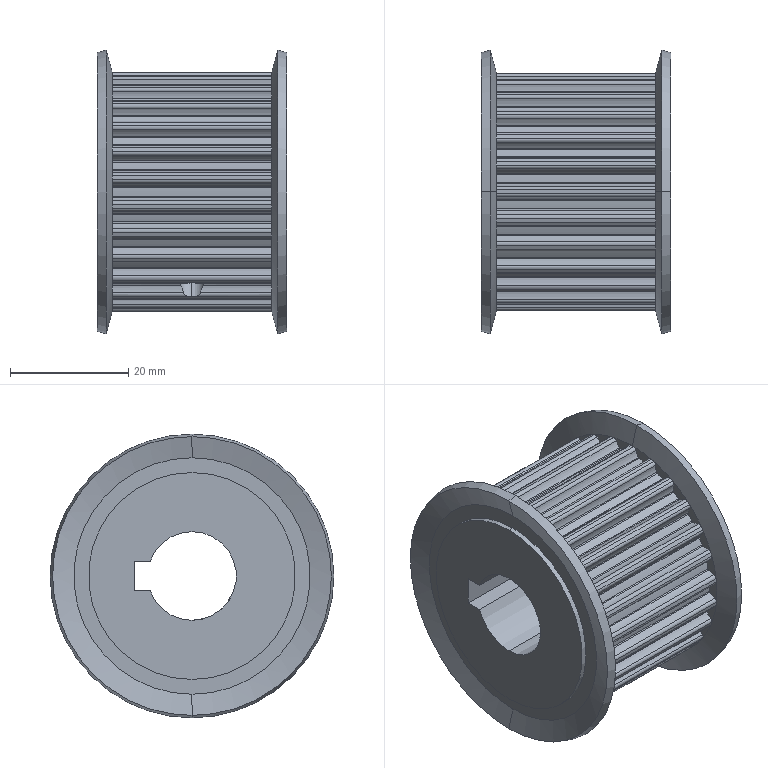Part | SolidWorks | features BaseBody 1 | 1 solid | 301 faces | box 32.122 x 48 x 48 mm | volume 32488 mm3 | cylinder 230 | plane 59 | cone 12 | commonest cylinder face diameters 0.5 x56 6.55 x56 1.1 x52 36.88 x28 40.42 x27 4.134 x4